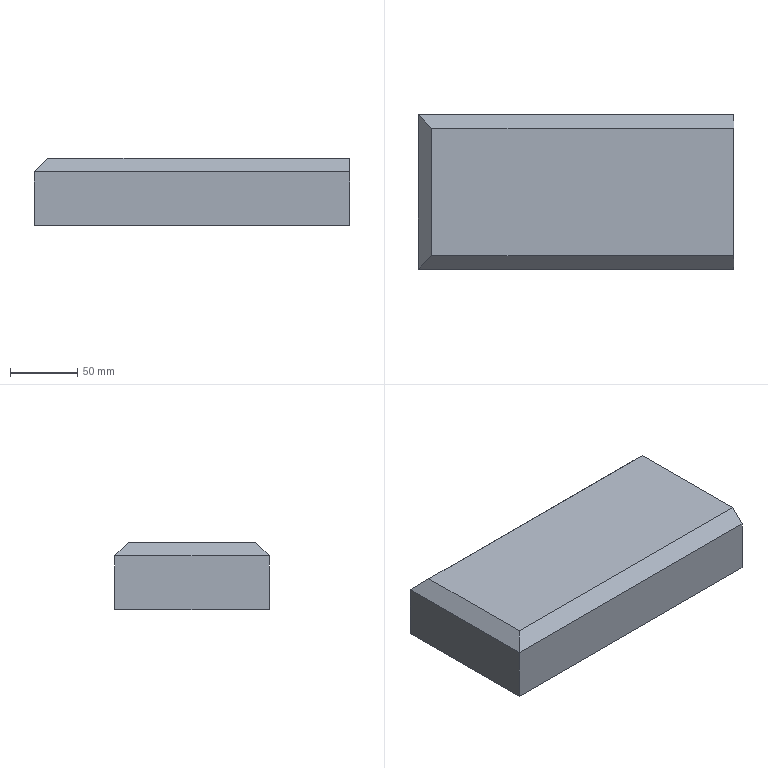Part | NX | features solid 2 | 1 solid | 9 faces | box 235 x 115 x 50 mm | volume 1322667 mm3 | plane 9
STEP:
#1=CARTESIAN_POINT('',(-55.,-135.,-270.));
#2=VERTEX_POINT('',#1);
#3=CARTESIAN_POINT('',(-55.,-230.,-270.));
#4=VERTEX_POINT('',#3);
#5=CARTESIAN_POINT('',(-55.,-125.,-270.));
#6=DIRECTION('',(0.,-1.,0.));
#7=VECTOR('',#6,1000.);
#8=LINE('',#5,#7);
#9=EDGE_CURVE('',#2,#4,#8,.T.);
#10=ORIENTED_EDGE('',*,*,#9,.F.);
#11=CARTESIAN_POINT('',(-280.,-135.,-270.));
#12=VERTEX_POINT('',#11);
#13=CARTESIAN_POINT('',(-290.,-135.,-270.));
#14=DIRECTION('',(-1.,0.,0.));
#15=VECTOR('',#14,1000.);
#16=LINE('',#13,#15);
#17=EDGE_CURVE('',#2,#12,#16,.T.);
#18=ORIENTED_EDGE('',*,*,#17,.T.);
#19=CARTESIAN_POINT('',(-280.,-230.,-270.));
#20=VERTEX_POINT('',#19);
#21=CARTESIAN_POINT('',(-280.,-125.,-270.));
#22=DIRECTION('',(0.,-1.,0.));
#23=VECTOR('',#22,1000.);
#24=LINE('',#21,#23);
#25=EDGE_CURVE('',#12,#20,#24,.T.);
#26=ORIENTED_EDGE('',*,*,#25,.T.);
#27=CARTESIAN_POINT('',(-55.,-230.,-270.));
#28=DIRECTION('',(1.,0.,0.));
#29=VECTOR('',#28,1000.);
#30=LINE('',#27,#29);
#31=EDGE_CURVE('',#20,#4,#30,.T.);
#32=ORIENTED_EDGE('',*,*,#31,.T.);
#33=EDGE_LOOP('',(#10,#18,#26,#32));
#34=FACE_BOUND('',#33,.T.);
#35=CARTESIAN_POINT('',(-290.,-125.,-270.));
#36=DIRECTION('',(0.,0.,1.));
#37=DIRECTION('',(1.,0.,0.));
#38=AXIS2_PLACEMENT_3D('',#35,#36,#37);
#39=PLANE('',#38);
#40=ADVANCED_FACE('',(#34),#39,.T.);
#41=CARTESIAN_POINT('',(-290.,-240.,-280.));
#42=VERTEX_POINT('',#41);
#43=CARTESIAN_POINT('',(-290.,-240.,-320.));
#44=VERTEX_POINT('',#43);
#45=CARTESIAN_POINT('',(-290.,-240.,-270.));
#46=DIRECTION('',(0.,0.,1.));
#47=VECTOR('',#46,1000.);
#48=LINE('',#45,#47);
#49=EDGE_CURVE('',#42,#44,#48,.F.);
#50=ORIENTED_EDGE('',*,*,#49,.F.);
#51=CARTESIAN_POINT('',(-290.,-125.,-280.));
#52=VERTEX_POINT('',#51);
#53=CARTESIAN_POINT('',(-290.,-125.,-280.));
#54=DIRECTION('',(0.,-1.,0.));
#55=VECTOR('',#54,1000.);
#56=LINE('',#53,#55);
#57=EDGE_CURVE('',#42,#52,#56,.F.);
#58=ORIENTED_EDGE('',*,*,#57,.T.);
#59=CARTESIAN_POINT('',(-290.,-125.,-320.));
#60=VERTEX_POINT('',#59);
#61=CARTESIAN_POINT('',(-290.,-125.,-270.));
#62=DIRECTION('',(0.,0.,-1.));
#63=VECTOR('',#62,1000.);
#64=LINE('',#61,#63);
#65=EDGE_CURVE('',#52,#60,#64,.T.);
#66=ORIENTED_EDGE('',*,*,#65,.T.);
#67=CARTESIAN_POINT('',(-290.,-125.,-320.));
#68=DIRECTION('',(0.,-1.,0.));
#69=VECTOR('',#68,1000.);
#70=LINE('',#67,#69);
#71=EDGE_CURVE('',#60,#44,#70,.T.);
#72=ORIENTED_EDGE('',*,*,#71,.T.);
#73=EDGE_LOOP('',(#50,#58,#66,#72));
#74=FACE_BOUND('',#73,.T.);
#75=CARTESIAN_POINT('',(-290.,-125.,-270.));
#76=DIRECTION('',(1.,0.,0.));
#77=DIRECTION('',(0.,0.,-1.));
#78=AXIS2_PLACEMENT_3D('',#75,#76,#77);
#79=PLANE('',#78);
#80=ADVANCED_FACE('',(#74),#79,.F.);
#81=ORIENTED_EDGE('',*,*,#71,.F.);
#82=CARTESIAN_POINT('',(-55.,-125.,-320.));
#83=VERTEX_POINT('',#82);
#84=CARTESIAN_POINT('',(-290.,-125.,-320.));
#85=DIRECTION('',(1.,0.,0.));
#86=VECTOR('',#85,1000.);
#87=LINE('',#84,#86);
#88=EDGE_CURVE('',#60,#83,#87,.T.);
#89=ORIENTED_EDGE('',*,*,#88,.T.);
#90=CARTESIAN_POINT('',(-55.,-240.,-320.));
#91=VERTEX_POINT('',#90);
#92=CARTESIAN_POINT('',(-55.,-125.,-320.));
#93=DIRECTION('',(0.,-1.,0.));
#94=VECTOR('',#93,1000.);
#95=LINE('',#92,#94);
#96=EDGE_CURVE('',#83,#91,#95,.T.);
#97=ORIENTED_EDGE('',*,*,#96,.T.);
#98=CARTESIAN_POINT('',(-290.,-240.,-320.));
#99=DIRECTION('',(1.,0.,0.));
#100=VECTOR('',#99,1000.);
#101=LINE('',#98,#100);
#102=EDGE_CURVE('',#44,#91,#101,.T.);
#103=ORIENTED_EDGE('',*,*,#102,.F.);
#104=EDGE_LOOP('',(#81,#89,#97,#103));
#105=FACE_BOUND('',#104,.T.);
#106=CARTESIAN_POINT('',(-290.,-125.,-320.));
#107=DIRECTION('',(0.,0.,1.));
#108=DIRECTION('',(1.,0.,0.));
#109=AXIS2_PLACEMENT_3D('',#106,#107,#108);
#110=PLANE('',#109);
#111=ADVANCED_FACE('',(#105),#110,.F.);
#112=CARTESIAN_POINT('',(-55.,-125.,-280.));
#113=VERTEX_POINT('',#112);
#114=CARTESIAN_POINT('',(-55.,-125.,-270.));
#115=DIRECTION('',(0.,0.,-1.));
#116=VECTOR('',#115,1000.);
#117=LINE('',#114,#116);
#118=EDGE_CURVE('',#113,#83,#117,.T.);
#119=ORIENTED_EDGE('',*,*,#118,.F.);
#120=CARTESIAN_POINT('',(-55.,-130.,-275.));
#121=DIRECTION('',(0.,0.7071,-0.7071));
#122=VECTOR('',#121,1000.);
#123=LINE('',#120,#122);
#124=EDGE_CURVE('',#113,#2,#123,.F.);
#125=ORIENTED_EDGE('',*,*,#124,.T.);
#126=ORIENTED_EDGE('',*,*,#9,.T.);
#127=CARTESIAN_POINT('',(-55.,-240.,-280.));
#128=VERTEX_POINT('',#127);
#129=CARTESIAN_POINT('',(-55.,-177.5,-217.5));
#130=DIRECTION('',(0.,-0.7071,-0.7071));
#131=VECTOR('',#130,1000.);
#132=LINE('',#129,#131);
#133=EDGE_CURVE('',#4,#128,#132,.T.);
#134=ORIENTED_EDGE('',*,*,#133,.T.);
#135=CARTESIAN_POINT('',(-55.,-240.,-270.));
#136=DIRECTION('',(0.,0.,1.));
#137=VECTOR('',#136,1000.);
#138=LINE('',#135,#137);
#139=EDGE_CURVE('',#128,#91,#138,.F.);
#140=ORIENTED_EDGE('',*,*,#139,.T.);
#141=ORIENTED_EDGE('',*,*,#96,.F.);
#142=EDGE_LOOP('',(#119,#125,#126,#134,#140,#141));
#143=FACE_BOUND('',#142,.T.);
#144=CARTESIAN_POINT('',(-55.,-125.,-270.));
#145=DIRECTION('',(1.,0.,0.));
#146=DIRECTION('',(0.,0.,-1.));
#147=AXIS2_PLACEMENT_3D('',#144,#145,#146);
#148=PLANE('',#147);
#149=ADVANCED_FACE('',(#143),#148,.T.);
#150=ORIENTED_EDGE('',*,*,#139,.F.);
#151=CARTESIAN_POINT('',(-290.,-240.,-280.));
#152=DIRECTION('',(-1.,0.,0.));
#153=VECTOR('',#152,1000.);
#154=LINE('',#151,#153);
#155=EDGE_CURVE('',#128,#42,#154,.T.);
#156=ORIENTED_EDGE('',*,*,#155,.T.);
#157=ORIENTED_EDGE('',*,*,#49,.T.);
#158=ORIENTED_EDGE('',*,*,#102,.T.);
#159=EDGE_LOOP('',(#150,#156,#157,#158));
#160=FACE_BOUND('',#159,.T.);
#161=CARTESIAN_POINT('',(-290.,-240.,-270.));
#162=DIRECTION('',(0.,1.,0.));
#163=DIRECTION('',(0.,0.,1.));
#164=AXIS2_PLACEMENT_3D('',#161,#162,#163);
#165=PLANE('',#164);
#166=ADVANCED_FACE('',(#160),#165,.F.);
#167=ORIENTED_EDGE('',*,*,#65,.F.);
#168=CARTESIAN_POINT('',(-290.,-125.,-280.));
#169=DIRECTION('',(1.,0.,0.));
#170=VECTOR('',#169,1000.);
#171=LINE('',#168,#170);
#172=EDGE_CURVE('',#52,#113,#171,.T.);
#173=ORIENTED_EDGE('',*,*,#172,.T.);
#174=ORIENTED_EDGE('',*,*,#118,.T.);
#175=ORIENTED_EDGE('',*,*,#88,.F.);
#176=EDGE_LOOP('',(#167,#173,#174,#175));
#177=FACE_BOUND('',#176,.T.);
#178=CARTESIAN_POINT('',(-290.,-125.,-270.));
#179=DIRECTION('',(0.,1.,0.));
#180=DIRECTION('',(0.,0.,1.));
#181=AXIS2_PLACEMENT_3D('',#178,#179,#180);
#182=PLANE('',#181);
#183=ADVANCED_FACE('',(#177),#182,.T.);
#184=ORIENTED_EDGE('',*,*,#133,.F.);
#185=ORIENTED_EDGE('',*,*,#31,.F.);
#186=CARTESIAN_POINT('',(-245.,-195.,-235.));
#187=DIRECTION('',(0.5774,0.5774,0.5774));
#188=VECTOR('',#187,1000.);
#189=LINE('',#186,#188);
#190=EDGE_CURVE('',#42,#20,#189,.T.);
#191=ORIENTED_EDGE('',*,*,#190,.F.);
#192=ORIENTED_EDGE('',*,*,#155,.F.);
#193=EDGE_LOOP('',(#184,#185,#191,#192));
#194=FACE_BOUND('',#193,.T.);
#195=CARTESIAN_POINT('',(-290.,-230.,-270.));
#196=DIRECTION('',(0.,-0.7071,0.7071));
#197=DIRECTION('',(-1.,0.,0.));
#198=AXIS2_PLACEMENT_3D('',#195,#196,#197);
#199=PLANE('',#198);
#200=ADVANCED_FACE('',(#194),#199,.T.);
#201=ORIENTED_EDGE('',*,*,#190,.T.);
#202=ORIENTED_EDGE('',*,*,#25,.F.);
#203=CARTESIAN_POINT('',(-283.333,-131.667,-273.333));
#204=DIRECTION('',(0.5774,-0.5774,0.5774));
#205=VECTOR('',#204,1000.);
#206=LINE('',#203,#205);
#207=EDGE_CURVE('',#52,#12,#206,.T.);
#208=ORIENTED_EDGE('',*,*,#207,.F.);
#209=ORIENTED_EDGE('',*,*,#57,.F.);
#210=EDGE_LOOP('',(#201,#202,#208,#209));
#211=FACE_BOUND('',#210,.T.);
#212=CARTESIAN_POINT('',(-280.,-125.,-270.));
#213=DIRECTION('',(-0.7071,0.,0.7071));
#214=DIRECTION('',(0.,1.,0.));
#215=AXIS2_PLACEMENT_3D('',#212,#213,#214);
#216=PLANE('',#215);
#217=ADVANCED_FACE('',(#211),#216,.T.);
#218=ORIENTED_EDGE('',*,*,#207,.T.);
#219=ORIENTED_EDGE('',*,*,#17,.F.);
#220=ORIENTED_EDGE('',*,*,#124,.F.);
#221=ORIENTED_EDGE('',*,*,#172,.F.);
#222=EDGE_LOOP('',(#218,#219,#220,#221));
#223=FACE_BOUND('',#222,.T.);
#224=CARTESIAN_POINT('',(-290.,-125.,-280.));
#225=DIRECTION('',(0.,-0.7071,-0.7071));
#226=DIRECTION('',(1.,0.,0.));
#227=AXIS2_PLACEMENT_3D('',#224,#225,#226);
#228=PLANE('',#227);
#229=ADVANCED_FACE('',(#223),#228,.F.);
#230=CLOSED_SHELL('',(#40,#80,#111,#149,#166,#183,#200,#217,#229));
#231=MANIFOLD_SOLID_BREP('',#230);
#232=(LENGTH_UNIT()NAMED_UNIT(*)SI_UNIT(.MILLI.,.METRE.));
#233=UNCERTAINTY_MEASURE_WITH_UNIT(LENGTH_MEASURE(0.00001),#232,'','');
#234=(NAMED_UNIT(*)PLANE_ANGLE_UNIT()SI_UNIT($,.RADIAN.));
#235=(NAMED_UNIT(*)SI_UNIT($,.STERADIAN.)SOLID_ANGLE_UNIT());
#236=(GEOMETRIC_REPRESENTATION_CONTEXT(3)GLOBAL_UNCERTAINTY_ASSIGNED_CONTEXT((#233))GLOBAL_UNIT_ASSIGNED_CONTEXT((#232,#234,#235))REPRESENTATION_CONTEXT('',''));
#237=ADVANCED_BREP_SHAPE_REPRESENTATION('',(#231),#236);